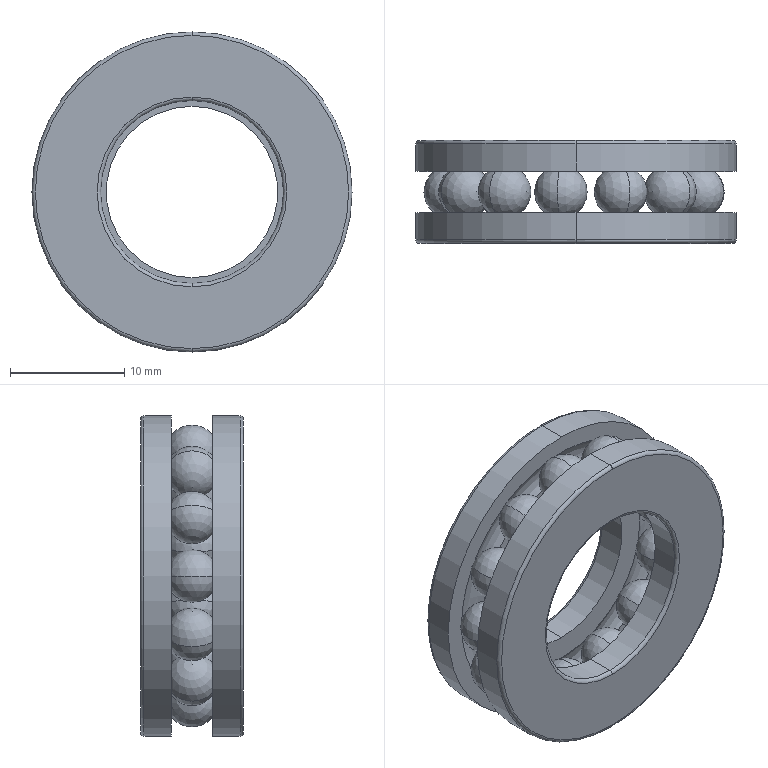Part | SolidWorks | features Revolution 3, CirPattern 1, Fillet 1 | 1 solid | 76 faces | box 28 x 9 x 28 mm | volume 2845 mm3 | torus 36 | sphere 26 | cylinder 8 | plane 6 | commonest cylinder face diameters 28 x4 15 x2 16 x2